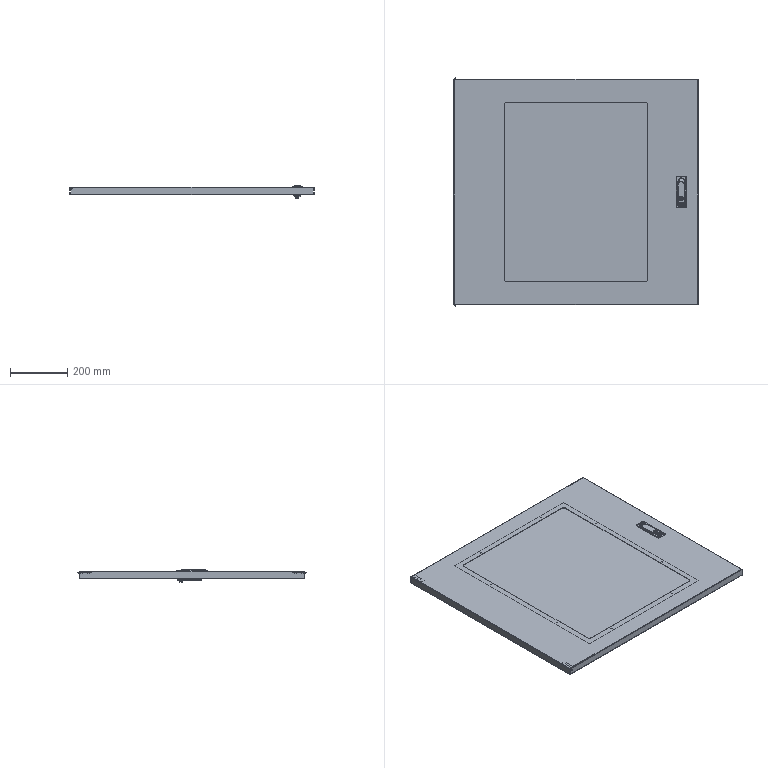Part | SolidWorks | 7 solids | 476 faces | box 851 x 799 x 42.5 mm | volume 2246546 mm3 | plane 256 | cylinder 180 | spline 28 | cone 12 | commonest cylinder face diameters 4 x50 3 x21 1 x17 2 x15 12 x8 8 x6